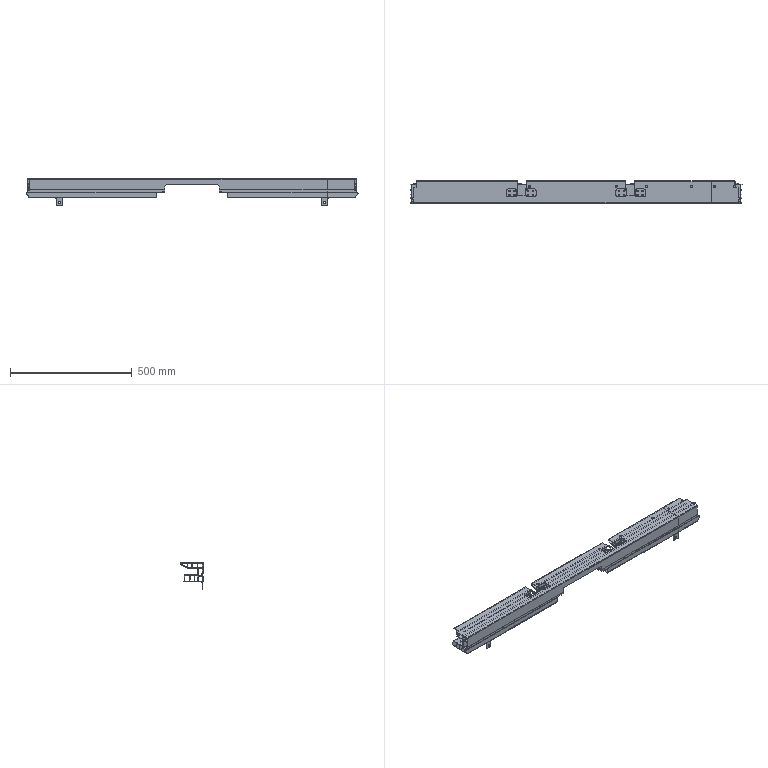CAM job | NX | 3+2 milling, drilling | part box 1365 x 90.95 x 108.501 mm
Tools:
number,name,description,diameter,corner_radius,flute_length,length,flutes
16,D16,Milling Tool-5 Parameters,16.0,0.0,50.0,75.0,2
10,D10,Milling Tool-5 Parameters,10.0,0.0,50.0,75.0,2
8,D8R0.5,Milling Tool-5 Parameters,8.0,0.5,50.0,75.0,2
7,D6A45,Milling Tool-5 Parameters,6.0,0.0,3.0,3.0,2
18,8.1ZT,Drilling Tool,8.0,0.0,35.0,50.0,2
17,7.1ZT,Drilling Tool,7.0,0.0,35.0,50.0,2
19,9.0ZT,Drilling Tool,9.0,0.0,35.0,50.0,2
14,6.6ZT,Drilling Tool,6.5,0.0,35.0,50.0,2
6,D6,Milling Tool-5 Parameters,6.0,0.0,50.0,75.0,2
9,R3,Milling Tool-5 Parameters,6.0,3.0,50.0,75.0,2
4,D4,Milling Tool-5 Parameters,4.0,0.0,50.0,75.0,2
Operations:
program,operation,operation_type,tool,method,geometry_group,spindle_rpm,surface_speed,feed_per_tooth,feed_cut,feed_plunge,cut_length_mm,path_length_mm,cut_time_min,machine_time_min
1,DRILLING_1,Operation,D6A45,METHOD,A,3500.0,65.0,0.0357,250.0,0.0,24.0,966.985,0.096,0.1903
1,DRILLING_COPY_3,Operation,8.1ZT,METHOD,A,1500.0,37.0,0.05,150.0,0.0,344.421,1607.826,2.296,2.422
1,CAVITY_MILL_1,CavityMilling,D16,METHOD,A,9500.0,477.0,0.1316,2500.0,1000.0,48369.55,51233.256,23.168,23.454
1,CAVITY_MILL_COPY,CavityMilling,D10,METHOD,A,6500.0,204.0,0.1385,1800.0,1000.0,4040.922,8148.374,2.824,3.234
1,FLOOR_WALL_1,VolumeBased25DMillingOperation,D10,METHOD,A,6000.0,188.0,0.0833,1000.0,100.0,1249.598,2176.932,1.25,1.342
1,ZLEVEL_PROFILE_COPY,ZLevelMilling,D10,METHOD,A,6000.0,301.0,0.1667,2000.0,100.0,750.865,3244.569,0.3754,0.6248
1,ZLEVEL_PROFILE_1_COPY_1_1,ZLevelMilling,D8R0.5,METHOD,A,6000.0,150.0,0.2083,2500.0,1000.0,46724.707,48985.601,18.701,18.927
1,CAVITY_MILL_COPY_COPY,CavityMilling,D4,METHOD,A,6500.0,204.0,0.1231,1600.0,1000.0,4401.053,7747.967,3.124,3.459
1,HOLE_MILLING_1_COPY,CylinderMilling,D4,METHOD,A,6000.0,113.0,0.1167,1400.0,100.0,902.287,2423.765,0.6445,0.7966
1,ZLEVEL_PROFILE_COPY_1_COPY_COPY_COPY_COPY_COPY,ZLevelMilling,D6A45,METHOD,A,6000.0,113.0,0.0833,1000.0,1000.0,846.619,5894.421,0.8466,1.351
2,CAVITY_MILL,CavityMilling,D16,METHOD,B,9500.0,477.0,0.1316,2500.0,1000.0,218256.77,256985.536,90.61,94.483
2,HOLE_MILLING,CylinderMilling,D16,METHOD,B,6000.0,301.0,0.1667,2000.0,100.0,6045.31,7597.31,3.023,3.178
2,DRILLING,Operation,D6A45,METHOD,B,3500.0,65.0,0.0357,250.0,0.0,88.0,1737.051,0.352,0.5169
2,DRILLING_COPY_1,Operation,D6A45,METHOD,B,3500.0,65.0,0.0357,250.0,0.0,4.0,239.0,0.016,0.0395
2,DRILLING_COPY,Operation,7.1ZT,METHOD,B,1500.0,37.0,0.05,150.0,0.0,36.412,1474.953,0.2427,0.3866
2,DRILLING_COPY_COPY,Operation,9.0ZT,METHOD,B,1500.0,37.0,0.05,150.0,0.0,155.262,1426.011,1.035,1.162
2,DRILLING_COPY_COPY_COPY,Operation,6.6ZT,METHOD,B,1500.0,37.0,0.05,150.0,0.0,8.953,248.906,0.0597,0.0837
2,FLOOR_WALL,VolumeBased25DMillingOperation,D10,METHOD,B,6000.0,188.0,0.0833,1000.0,100.0,29006.299,30322.397,29.006,29.138
2,FLOOR_WALL_COPY,VolumeBased25DMillingOperation,D10,METHOD,B,6000.0,188.0,0.0833,1000.0,100.0,2343.113,6559.961,2.343,2.765
2,11,ZLevelMilling,D10,METHOD,B,5500.0,138.0,0.0909,1000.0,500.0,199.78,1855.991,0.2445,0.4101
2,11_COPY,ZLevelMilling,D10,METHOD,B,5500.0,138.0,0.0909,1000.0,500.0,301.829,1035.053,0.3242,0.3975
2,ZLEVEL_PROFILE_1,ZLevelMilling,D8R0.5,METHOD,B,6000.0,150.0,0.2083,2500.0,1000.0,1526.464,3103.547,0.6192,0.7769
2,ZLEVEL_PROFILE_1_COPY,ZLevelMilling,D8R0.5,METHOD,B,6000.0,150.0,0.2083,2500.0,1000.0,882.625,2247.474,0.3615,0.498
2,ZLEVEL_PROFILE_1_COPY_COPY,ZLevelMilling,D8R0.5,METHOD,B,6000.0,150.0,0.2083,2500.0,1000.0,2975.203,4088.298,1.199,1.31
2,ZLEVEL_PROFILE_1_COPY_1,ZLevelMilling,D8R0.5,METHOD,B,6000.0,150.0,0.2083,2500.0,1000.0,49844.176,52649.088,19.955,20.235
2,ZLEVEL_PROFILE_COPY_1_COPY_COPY_COPY_COPY,ZLevelMilling,D6A45,METHOD,B,6000.0,113.0,0.0833,1000.0,1000.0,1946.507,10206.516,1.946,2.772
2,TOOL16,CylinderMilling,D16,METHOD,B,6000.0,301.0,0.1,1200.0,100.0,1389.012,2883.412,1.157,1.307
3,FLOOR_WALL_COPY_COPY,VolumeBased25DMillingOperation,D10,METHOD,C,6000.0,188.0,0.2083,2500.0,1000.0,74767.144,108678.829,39.81,43.202
3,FLOOR_WALL_COPY_COPY_COPY,VolumeBased25DMillingOperation,D10,METHOD,C,6000.0,188.0,0.1,1200.0,1000.0,1425.329,3840.747,1.357,1.599
3,FLOOR_WALL_COPY_COPY_COPY_COPY,VolumeBased25DMillingOperation,D10,METHOD,C,6000.0,188.0,0.1,1200.0,1000.0,1119.118,5024.38,0.9583,1.349
3,FLOOR_WALL_COPY_COPY_COPY_1,VolumeBased25DMillingOperation,D10,METHOD,C,6000.0,188.0,0.0833,1000.0,1000.0,1779.645,5371.089,1.78,2.139
3,FLOOR_WALL_COPY_COPY_COPY_1_COPY,VolumeBased25DMillingOperation,D10,METHOD,C,6000.0,188.0,0.0833,1000.0,1000.0,466.47,1193.028,0.4665,0.5391
3,FIXED_CONTOUR_COPY,SurfaceContour,D6,METHOD,C,9500.0,179.0,0.1316,2500.0,1000.0,947.725,2140.953,0.3843,0.5037
3,FIXED_CONTOUR,SurfaceContour,R3,METHOD,C,9500.0,179.0,0.1316,2500.0,1000.0,456.596,1661.842,0.1884,0.3089
3,DRILLING_COPY_2,Operation,D6A45,METHOD,C,3500.0,65.0,0.0357,250.0,0.0,16.0,1472.028,0.064,0.2096
3,DRILLING_COPY_COPY_1,Operation,7.1ZT,METHOD,C,1500.0,37.0,0.05,150.0,0.0,17.206,1467.917,0.1147,0.2598
3,DRILLING_COPY_COPY_1_COPY,Operation,7.1ZT,METHOD,C,1500.0,37.0,0.05,150.0,0.0,54.206,1501.816,0.3614,0.5061
3,HOLE_MILLING_COPY,CylinderMilling,D10,METHOD,C,6000.0,301.0,0.1667,2000.0,100.0,258.934,1767.634,0.1295,0.2803
3,11_COPY_1,ZLevelMilling,D10,METHOD,C,5500.0,138.0,0.0909,1000.0,500.0,415.786,1262.887,0.4604,0.5451
3,ZLEVEL_PROFILE_1_COPY_1_COPY,ZLevelMilling,D8R0.5,METHOD,C,6000.0,150.0,0.2083,2500.0,1000.0,12003.659,15767.351,4.827,5.204
4,HOLE_MILLING_1_COPY_2,CylinderMilling,D6,METHOD,D,6000.0,113.0,0.1167,1400.0,100.0,152.405,1368.605,0.1089,0.2305
4,ZLEVEL_PROFILE_COPY_1_COPY_COPY_COPY_COPY_COPY_1,ZLevelMilling,D6A45,METHOD,D,6000.0,113.0,0.0833,1000.0,1000.0,38.123,1254.698,0.0381,0.1598